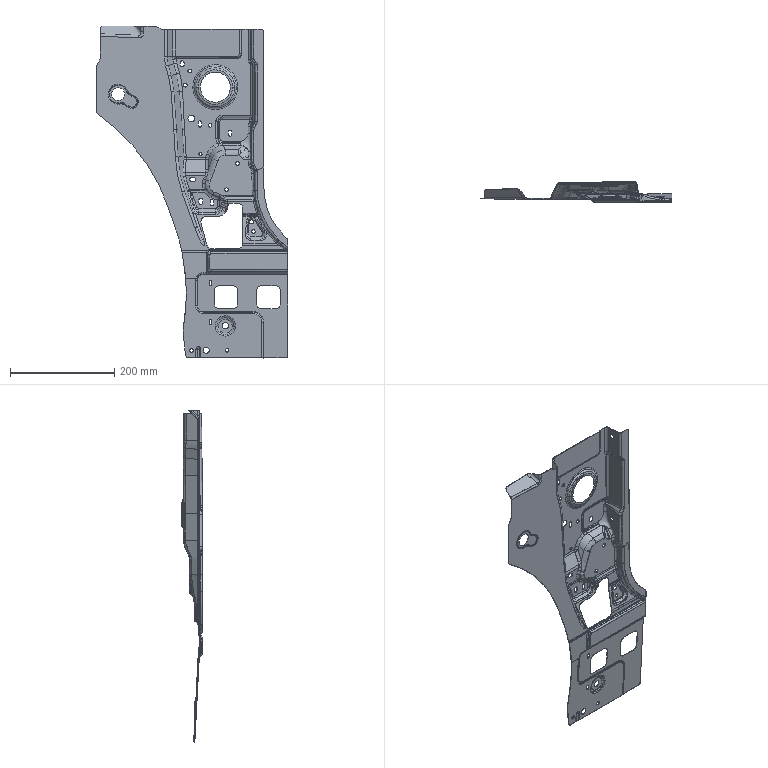Part | STEP file | FNA5401331 | 1 solid | 868 faces | box 367 x 39.355 x 636.857 mm | volume 124897 mm3 | spline 513 | cylinder 236 | plane 110 | other 7 | sphere 2 | commonest cylinder face diameters 6 x28 7 x28 12 x26 20 x15 4.4 x13 7.6 x13